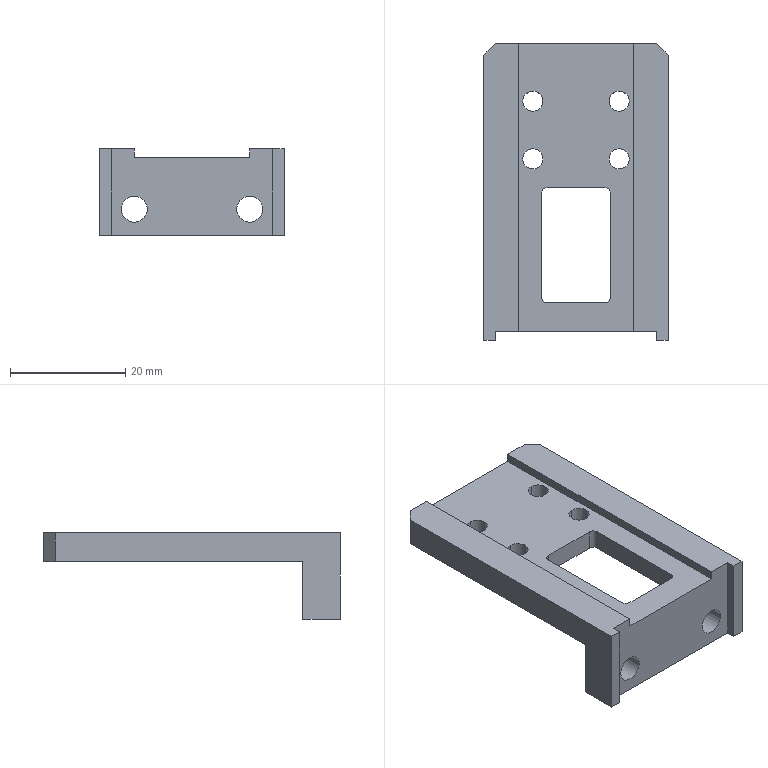Part | STEP file | 11-FG-E04211 | 1 solid | 37 faces | box 32 x 51.5 x 15 mm | volume 7039 mm3 | plane 21 | cylinder 16 | commonest cylinder face diameters 3.5 x8 2 x4 4.5 x4
STEP:
#1=CARTESIAN_POINT('',(12.25,-25.,4.5));
#2=VERTEX_POINT('',#1);
#3=CARTESIAN_POINT('',(7.75,-25.,4.5));
#4=VERTEX_POINT('',#3);
#5=CARTESIAN_POINT('',(10.,-25.,4.5));
#6=DIRECTION('',(0.,1.,0.));
#7=DIRECTION('',(0.,0.,1.));
#8=AXIS2_PLACEMENT_3D('',#5,#6,#7);
#9=CIRCLE('',#8,2.25);
#10=EDGE_CURVE('',#2,#4,#9,.T.);
#11=ORIENTED_EDGE('',*,*,#10,.F.);
#12=CARTESIAN_POINT('',(12.25,-20.,4.5));
#13=VERTEX_POINT('',#12);
#14=CARTESIAN_POINT('',(12.25,-30.,4.5));
#15=DIRECTION('',(0.,1.,0.));
#16=VECTOR('',#15,1000.);
#17=LINE('',#14,#16);
#18=EDGE_CURVE('',#2,#13,#17,.T.);
#19=ORIENTED_EDGE('',*,*,#18,.T.);
#20=CARTESIAN_POINT('',(7.75,-20.,4.5));
#21=VERTEX_POINT('',#20);
#22=CARTESIAN_POINT('',(10.,-20.,4.5));
#23=DIRECTION('',(0.,1.,0.));
#24=DIRECTION('',(-1.,0.,0.));
#25=AXIS2_PLACEMENT_3D('',#22,#23,#24);
#26=CIRCLE('',#25,2.25);
#27=EDGE_CURVE('',#13,#21,#26,.T.);
#28=ORIENTED_EDGE('',*,*,#27,.T.);
#29=CARTESIAN_POINT('',(7.75,-30.,4.5));
#30=DIRECTION('',(0.,1.,0.));
#31=VECTOR('',#30,1000.);
#32=LINE('',#29,#31);
#33=EDGE_CURVE('',#4,#21,#32,.T.);
#34=ORIENTED_EDGE('',*,*,#33,.F.);
#35=EDGE_LOOP('',(#11,#19,#28,#34));
#36=FACE_OUTER_BOUND('',#35,.T.);
#37=CARTESIAN_POINT('',(10.,-30.,4.5));
#38=DIRECTION('',(0.,1.,0.));
#39=DIRECTION('',(-1.,0.,0.));
#40=AXIS2_PLACEMENT_3D('',#37,#38,#39);
#41=CYLINDRICAL_SURFACE('',#40,2.25);
#42=ADVANCED_FACE('',(#36),#41,.F.);
#43=CARTESIAN_POINT('',(-7.75,-25.,4.5));
#44=VERTEX_POINT('',#43);
#45=CARTESIAN_POINT('',(-12.25,-25.,4.5));
#46=VERTEX_POINT('',#45);
#47=CARTESIAN_POINT('',(-10.,-25.,4.5));
#48=DIRECTION('',(0.,1.,0.));
#49=DIRECTION('',(0.,0.,1.));
#50=AXIS2_PLACEMENT_3D('',#47,#48,#49);
#51=CIRCLE('',#50,2.25);
#52=EDGE_CURVE('',#44,#46,#51,.T.);
#53=ORIENTED_EDGE('',*,*,#52,.F.);
#54=CARTESIAN_POINT('',(-7.75,-20.,4.5));
#55=VERTEX_POINT('',#54);
#56=CARTESIAN_POINT('',(-7.75,-30.,4.5));
#57=DIRECTION('',(0.,1.,0.));
#58=VECTOR('',#57,1000.);
#59=LINE('',#56,#58);
#60=EDGE_CURVE('',#44,#55,#59,.T.);
#61=ORIENTED_EDGE('',*,*,#60,.T.);
#62=CARTESIAN_POINT('',(-12.25,-20.,4.5));
#63=VERTEX_POINT('',#62);
#64=CARTESIAN_POINT('',(-10.,-20.,4.5));
#65=DIRECTION('',(0.,1.,0.));
#66=DIRECTION('',(-1.,0.,0.));
#67=AXIS2_PLACEMENT_3D('',#64,#65,#66);
#68=CIRCLE('',#67,2.25);
#69=EDGE_CURVE('',#55,#63,#68,.T.);
#70=ORIENTED_EDGE('',*,*,#69,.T.);
#71=CARTESIAN_POINT('',(-12.25,-30.,4.5));
#72=DIRECTION('',(0.,1.,0.));
#73=VECTOR('',#72,1000.);
#74=LINE('',#71,#73);
#75=EDGE_CURVE('',#46,#63,#74,.T.);
#76=ORIENTED_EDGE('',*,*,#75,.F.);
#77=EDGE_LOOP('',(#53,#61,#70,#76));
#78=FACE_OUTER_BOUND('',#77,.T.);
#79=CARTESIAN_POINT('',(-10.,-30.,4.5));
#80=DIRECTION('',(0.,1.,0.));
#81=DIRECTION('',(-1.,0.,0.));
#82=AXIS2_PLACEMENT_3D('',#79,#80,#81);
#83=CYLINDRICAL_SURFACE('',#82,2.25);
#84=ADVANCED_FACE('',(#78),#83,.F.);
#85=CARTESIAN_POINT('',(-7.5,13.25,13.5));
#86=VERTEX_POINT('',#85);
#87=CARTESIAN_POINT('',(-7.5,16.75,13.5));
#88=VERTEX_POINT('',#87);
#89=CARTESIAN_POINT('',(-7.5,15.,13.5));
#90=DIRECTION('',(0.,0.,-1.));
#91=DIRECTION('',(-1.,0.,0.));
#92=AXIS2_PLACEMENT_3D('',#89,#90,#91);
#93=CIRCLE('',#92,1.75);
#94=EDGE_CURVE('',#86,#88,#93,.T.);
#95=ORIENTED_EDGE('',*,*,#94,.F.);
#96=CARTESIAN_POINT('',(-7.5,13.25,10.));
#97=VERTEX_POINT('',#96);
#98=CARTESIAN_POINT('',(-7.5,13.25,161.));
#99=DIRECTION('',(0.,0.,-1.));
#100=VECTOR('',#99,1000.);
#101=LINE('',#98,#100);
#102=EDGE_CURVE('',#86,#97,#101,.T.);
#103=ORIENTED_EDGE('',*,*,#102,.T.);
#104=CARTESIAN_POINT('',(-7.5,16.75,10.));
#105=VERTEX_POINT('',#104);
#106=CARTESIAN_POINT('',(-7.5,15.,10.));
#107=DIRECTION('',(0.,0.,-1.));
#108=DIRECTION('',(0.,1.,0.));
#109=AXIS2_PLACEMENT_3D('',#106,#107,#108);
#110=CIRCLE('',#109,1.75);
#111=EDGE_CURVE('',#97,#105,#110,.T.);
#112=ORIENTED_EDGE('',*,*,#111,.T.);
#113=CARTESIAN_POINT('',(-7.5,16.75,161.));
#114=DIRECTION('',(0.,0.,-1.));
#115=VECTOR('',#114,1000.);
#116=LINE('',#113,#115);
#117=EDGE_CURVE('',#88,#105,#116,.T.);
#118=ORIENTED_EDGE('',*,*,#117,.F.);
#119=EDGE_LOOP('',(#95,#103,#112,#118));
#120=FACE_OUTER_BOUND('',#119,.T.);
#121=CARTESIAN_POINT('',(-7.5,15.,161.));
#122=DIRECTION('',(0.,0.,-1.));
#123=DIRECTION('',(0.,1.,0.));
#124=AXIS2_PLACEMENT_3D('',#121,#122,#123);
#125=CYLINDRICAL_SURFACE('',#124,1.75);
#126=ADVANCED_FACE('',(#120),#125,.F.);
#127=CARTESIAN_POINT('',(7.5,3.25,13.5));
#128=VERTEX_POINT('',#127);
#129=CARTESIAN_POINT('',(7.5,6.75,13.5));
#130=VERTEX_POINT('',#129);
#131=CARTESIAN_POINT('',(7.5,5.,13.5));
#132=DIRECTION('',(0.,0.,-1.));
#133=DIRECTION('',(-1.,0.,0.));
#134=AXIS2_PLACEMENT_3D('',#131,#132,#133);
#135=CIRCLE('',#134,1.75);
#136=EDGE_CURVE('',#128,#130,#135,.T.);
#137=ORIENTED_EDGE('',*,*,#136,.F.);
#138=CARTESIAN_POINT('',(7.5,3.25,10.));
#139=VERTEX_POINT('',#138);
#140=CARTESIAN_POINT('',(7.5,3.25,161.));
#141=DIRECTION('',(0.,0.,-1.));
#142=VECTOR('',#141,1000.);
#143=LINE('',#140,#142);
#144=EDGE_CURVE('',#128,#139,#143,.T.);
#145=ORIENTED_EDGE('',*,*,#144,.T.);
#146=CARTESIAN_POINT('',(7.5,6.75,10.));
#147=VERTEX_POINT('',#146);
#148=CARTESIAN_POINT('',(7.5,5.,10.));
#149=DIRECTION('',(0.,0.,-1.));
#150=DIRECTION('',(0.,1.,0.));
#151=AXIS2_PLACEMENT_3D('',#148,#149,#150);
#152=CIRCLE('',#151,1.75);
#153=EDGE_CURVE('',#139,#147,#152,.T.);
#154=ORIENTED_EDGE('',*,*,#153,.T.);
#155=CARTESIAN_POINT('',(7.5,6.75,161.));
#156=DIRECTION('',(0.,0.,-1.));
#157=VECTOR('',#156,1000.);
#158=LINE('',#155,#157);
#159=EDGE_CURVE('',#130,#147,#158,.T.);
#160=ORIENTED_EDGE('',*,*,#159,.F.);
#161=EDGE_LOOP('',(#137,#145,#154,#160));
#162=FACE_OUTER_BOUND('',#161,.T.);
#163=CARTESIAN_POINT('',(7.5,5.,161.));
#164=DIRECTION('',(0.,0.,-1.));
#165=DIRECTION('',(0.,1.,0.));
#166=AXIS2_PLACEMENT_3D('',#163,#164,#165);
#167=CYLINDRICAL_SURFACE('',#166,1.75);
#168=ADVANCED_FACE('',(#162),#167,.F.);
#169=CARTESIAN_POINT('',(-7.5,3.25,13.5));
#170=VERTEX_POINT('',#169);
#171=CARTESIAN_POINT('',(-7.5,6.75,13.5));
#172=VERTEX_POINT('',#171);
#173=CARTESIAN_POINT('',(-7.5,5.,13.5));
#174=DIRECTION('',(0.,0.,-1.));
#175=DIRECTION('',(-1.,0.,0.));
#176=AXIS2_PLACEMENT_3D('',#173,#174,#175);
#177=CIRCLE('',#176,1.75);
#178=EDGE_CURVE('',#170,#172,#177,.T.);
#179=ORIENTED_EDGE('',*,*,#178,.F.);
#180=CARTESIAN_POINT('',(-7.5,3.25,10.));
#181=VERTEX_POINT('',#180);
#182=CARTESIAN_POINT('',(-7.5,3.25,161.));
#183=DIRECTION('',(0.,0.,-1.));
#184=VECTOR('',#183,1000.);
#185=LINE('',#182,#184);
#186=EDGE_CURVE('',#170,#181,#185,.T.);
#187=ORIENTED_EDGE('',*,*,#186,.T.);
#188=CARTESIAN_POINT('',(-7.5,6.75,10.));
#189=VERTEX_POINT('',#188);
#190=CARTESIAN_POINT('',(-7.5,5.,10.));
#191=DIRECTION('',(0.,0.,-1.));
#192=DIRECTION('',(0.,1.,0.));
#193=AXIS2_PLACEMENT_3D('',#190,#191,#192);
#194=CIRCLE('',#193,1.75);
#195=EDGE_CURVE('',#181,#189,#194,.T.);
#196=ORIENTED_EDGE('',*,*,#195,.T.);
#197=CARTESIAN_POINT('',(-7.5,6.75,161.));
#198=DIRECTION('',(0.,0.,-1.));
#199=VECTOR('',#198,1000.);
#200=LINE('',#197,#199);
#201=EDGE_CURVE('',#172,#189,#200,.T.);
#202=ORIENTED_EDGE('',*,*,#201,.F.);
#203=EDGE_LOOP('',(#179,#187,#196,#202));
#204=FACE_OUTER_BOUND('',#203,.T.);
#205=CARTESIAN_POINT('',(-7.5,5.,161.));
#206=DIRECTION('',(0.,0.,-1.));
#207=DIRECTION('',(0.,1.,0.));
#208=AXIS2_PLACEMENT_3D('',#205,#206,#207);
#209=CYLINDRICAL_SURFACE('',#208,1.75);
#210=ADVANCED_FACE('',(#204),#209,.F.);
#211=CARTESIAN_POINT('',(7.5,13.25,13.5));
#212=VERTEX_POINT('',#211);
#213=CARTESIAN_POINT('',(7.5,16.75,13.5));
#214=VERTEX_POINT('',#213);
#215=CARTESIAN_POINT('',(7.5,15.,13.5));
#216=DIRECTION('',(0.,0.,-1.));
#217=DIRECTION('',(-1.,0.,0.));
#218=AXIS2_PLACEMENT_3D('',#215,#216,#217);
#219=CIRCLE('',#218,1.75);
#220=EDGE_CURVE('',#212,#214,#219,.T.);
#221=ORIENTED_EDGE('',*,*,#220,.F.);
#222=CARTESIAN_POINT('',(7.5,13.25,10.));
#223=VERTEX_POINT('',#222);
#224=CARTESIAN_POINT('',(7.5,13.25,161.));
#225=DIRECTION('',(0.,0.,-1.));
#226=VECTOR('',#225,1000.);
#227=LINE('',#224,#226);
#228=EDGE_CURVE('',#212,#223,#227,.T.);
#229=ORIENTED_EDGE('',*,*,#228,.T.);
#230=CARTESIAN_POINT('',(7.5,16.75,10.));
#231=VERTEX_POINT('',#230);
#232=CARTESIAN_POINT('',(7.5,15.,10.));
#233=DIRECTION('',(0.,0.,-1.));
#234=DIRECTION('',(0.,1.,0.));
#235=AXIS2_PLACEMENT_3D('',#232,#233,#234);
#236=CIRCLE('',#235,1.75);
#237=EDGE_CURVE('',#223,#231,#236,.T.);
#238=ORIENTED_EDGE('',*,*,#237,.T.);
#239=CARTESIAN_POINT('',(7.5,16.75,161.));
#240=DIRECTION('',(0.,0.,-1.));
#241=VECTOR('',#240,1000.);
#242=LINE('',#239,#241);
#243=EDGE_CURVE('',#214,#231,#242,.T.);
#244=ORIENTED_EDGE('',*,*,#243,.F.);
#245=EDGE_LOOP('',(#221,#229,#238,#244));
#246=FACE_OUTER_BOUND('',#245,.T.);
#247=CARTESIAN_POINT('',(7.5,15.,161.));
#248=DIRECTION('',(0.,0.,-1.));
#249=DIRECTION('',(0.,1.,0.));
#250=AXIS2_PLACEMENT_3D('',#247,#248,#249);
#251=CYLINDRICAL_SURFACE('',#250,1.75);
#252=ADVANCED_FACE('',(#246),#251,.F.);
#253=CARTESIAN_POINT('',(10.,-25.,4.5));
#254=DIRECTION('',(0.,1.,0.));
#255=DIRECTION('',(0.,0.,1.));
#256=AXIS2_PLACEMENT_3D('',#253,#254,#255);
#257=CIRCLE('',#256,2.25);
#258=EDGE_CURVE('',#4,#2,#257,.T.);
#259=ORIENTED_EDGE('',*,*,#258,.T.);
#260=ORIENTED_EDGE('',*,*,#10,.T.);
#261=EDGE_LOOP('',(#259,#260));
#262=FACE_BOUND('',#261,.T.);
#263=CARTESIAN_POINT('',(-10.,-25.,4.5));
#264=DIRECTION('',(0.,1.,0.));
#265=DIRECTION('',(0.,0.,1.));
#266=AXIS2_PLACEMENT_3D('',#263,#264,#265);
#267=CIRCLE('',#266,2.25);
#268=EDGE_CURVE('',#46,#44,#267,.T.);
#269=ORIENTED_EDGE('',*,*,#268,.T.);
#270=ORIENTED_EDGE('',*,*,#52,.T.);
#271=EDGE_LOOP('',(#269,#270));
#272=FACE_BOUND('',#271,.T.);
#273=CARTESIAN_POINT('',(-14.,-25.,15.));
#274=VERTEX_POINT('',#273);
#275=CARTESIAN_POINT('',(-10.,-25.,15.));
#276=VERTEX_POINT('',#275);
#277=CARTESIAN_POINT('',(-16.,-25.,15.));
#278=DIRECTION('',(1.,0.,0.));
#279=VECTOR('',#278,1000.);
#280=LINE('',#277,#279);
#281=EDGE_CURVE('',#274,#276,#280,.T.);
#282=ORIENTED_EDGE('',*,*,#281,.F.);
#283=CARTESIAN_POINT('',(-14.,-25.,0.));
#284=VERTEX_POINT('',#283);
#285=CARTESIAN_POINT('',(-14.,-25.,17.5));
#286=DIRECTION('',(0.,0.,-1.));
#287=VECTOR('',#286,1000.);
#288=LINE('',#285,#287);
#289=EDGE_CURVE('',#274,#284,#288,.T.);
#290=ORIENTED_EDGE('',*,*,#289,.T.);
#291=CARTESIAN_POINT('',(14.,-25.,0.));
#292=VERTEX_POINT('',#291);
#293=CARTESIAN_POINT('',(-16.,-25.,0.));
#294=DIRECTION('',(1.,0.,0.));
#295=VECTOR('',#294,1000.);
#296=LINE('',#293,#295);
#297=EDGE_CURVE('',#284,#292,#296,.T.);
#298=ORIENTED_EDGE('',*,*,#297,.T.);
#299=CARTESIAN_POINT('',(14.,-25.,15.));
#300=VERTEX_POINT('',#299);
#301=CARTESIAN_POINT('',(14.,-25.,17.5));
#302=DIRECTION('',(0.,0.,-1.));
#303=VECTOR('',#302,1000.);
#304=LINE('',#301,#303);
#305=EDGE_CURVE('',#300,#292,#304,.T.);
#306=ORIENTED_EDGE('',*,*,#305,.F.);
#307=CARTESIAN_POINT('',(10.,-25.,15.));
#308=VERTEX_POINT('',#307);
#309=CARTESIAN_POINT('',(-16.,-25.,15.));
#310=DIRECTION('',(1.,0.,0.));
#311=VECTOR('',#310,1000.);
#312=LINE('',#309,#311);
#313=EDGE_CURVE('',#308,#300,#312,.T.);
#314=ORIENTED_EDGE('',*,*,#313,.F.);
#315=CARTESIAN_POINT('',(10.,-25.,13.5));
#316=VERTEX_POINT('',#315);
#317=CARTESIAN_POINT('',(10.,-25.,15.));
#318=DIRECTION('',(0.,0.,-1.));
#319=VECTOR('',#318,1000.);
#320=LINE('',#317,#319);
#321=EDGE_CURVE('',#308,#316,#320,.T.);
#322=ORIENTED_EDGE('',*,*,#321,.T.);
#323=CARTESIAN_POINT('',(-10.,-25.,13.5));
#324=VERTEX_POINT('',#323);
#325=CARTESIAN_POINT('',(-16.,-25.,13.5));
#326=DIRECTION('',(-1.,0.,0.));
#327=VECTOR('',#326,1000.);
#328=LINE('',#325,#327);
#329=EDGE_CURVE('',#316,#324,#328,.T.);
#330=ORIENTED_EDGE('',*,*,#329,.T.);
#331=CARTESIAN_POINT('',(-10.,-25.,15.));
#332=DIRECTION('',(0.,0.,1.));
#333=VECTOR('',#332,1000.);
#334=LINE('',#331,#333);
#335=EDGE_CURVE('',#324,#276,#334,.T.);
#336=ORIENTED_EDGE('',*,*,#335,.T.);
#337=EDGE_LOOP('',(#282,#290,#298,#306,#314,#322,#330,#336));
#338=FACE_OUTER_BOUND('',#337,.T.);
#339=CARTESIAN_POINT('',(-16.,-25.,15.));
#340=DIRECTION('',(0.,1.,0.));
#341=DIRECTION('',(0.,0.,1.));
#342=AXIS2_PLACEMENT_3D('',#339,#340,#341);
#343=PLANE('',#342);
#344=ADVANCED_FACE('',(#262,#272,#338),#343,.F.);
#345=CARTESIAN_POINT('',(16.,-26.5,15.));
#346=VERTEX_POINT('',#345);
#347=CARTESIAN_POINT('',(16.,23.,15.));
#348=VERTEX_POINT('',#347);
#349=CARTESIAN_POINT('',(16.,25.,15.));
#350=DIRECTION('',(0.,1.,0.));
#351=VECTOR('',#350,1000.);
#352=LINE('',#349,#351);
#353=EDGE_CURVE('',#346,#348,#352,.T.);
#354=ORIENTED_EDGE('',*,*,#353,.T.);
#355=CARTESIAN_POINT('',(14.,25.,15.));
#356=VERTEX_POINT('',#355);
#357=CARTESIAN_POINT('',(19.5,19.5,15.));
#358=DIRECTION('',(-0.7071,0.7071,0.));
#359=VECTOR('',#358,1000.);
#360=LINE('',#357,#359);
#361=EDGE_CURVE('',#348,#356,#360,.T.);
#362=ORIENTED_EDGE('',*,*,#361,.T.);
#363=CARTESIAN_POINT('',(10.,25.,15.));
#364=VERTEX_POINT('',#363);
#365=CARTESIAN_POINT('',(-16.,25.,15.));
#366=DIRECTION('',(-1.,0.,0.));
#367=VECTOR('',#366,1000.);
#368=LINE('',#365,#367);
#369=EDGE_CURVE('',#356,#364,#368,.T.);
#370=ORIENTED_EDGE('',*,*,#369,.T.);
#371=CARTESIAN_POINT('',(10.,0.,15.));
#372=DIRECTION('',(0.,1.,0.));
#373=VECTOR('',#372,1000.);
#374=LINE('',#371,#373);
#375=EDGE_CURVE('',#308,#364,#374,.T.);
#376=ORIENTED_EDGE('',*,*,#375,.F.);
#377=ORIENTED_EDGE('',*,*,#313,.T.);
#378=CARTESIAN_POINT('',(14.,-26.5,15.));
#379=VERTEX_POINT('',#378);
#380=CARTESIAN_POINT('',(14.,-25.,15.));
#381=DIRECTION('',(0.,1.,0.));
#382=VECTOR('',#381,1000.);
#383=LINE('',#380,#382);
#384=EDGE_CURVE('',#379,#300,#383,.T.);
#385=ORIENTED_EDGE('',*,*,#384,.F.);
#386=CARTESIAN_POINT('',(16.,-26.5,15.));
#387=DIRECTION('',(-1.,0.,0.));
#388=VECTOR('',#387,1000.);
#389=LINE('',#386,#388);
#390=EDGE_CURVE('',#346,#379,#389,.T.);
#391=ORIENTED_EDGE('',*,*,#390,.F.);
#392=EDGE_LOOP('',(#354,#362,#370,#376,#377,#385,#391));
#393=FACE_OUTER_BOUND('',#392,.T.);
#394=CARTESIAN_POINT('',(0.,0.,15.));
#395=DIRECTION('',(0.,0.,1.));
#396=DIRECTION('',(1.,0.,0.));
#397=AXIS2_PLACEMENT_3D('',#394,#395,#396);
#398=PLANE('',#397);
#399=ADVANCED_FACE('',(#393),#398,.T.);
#400=CARTESIAN_POINT('',(16.,-20.,10.));
#401=VERTEX_POINT('',#400);
#402=CARTESIAN_POINT('',(16.,23.,10.));
#403=VERTEX_POINT('',#402);
#404=CARTESIAN_POINT('',(16.,25.,10.));
#405=DIRECTION('',(0.,1.,0.));
#406=VECTOR('',#405,1000.);
#407=LINE('',#404,#406);
#408=EDGE_CURVE('',#401,#403,#407,.T.);
#409=ORIENTED_EDGE('',*,*,#408,.T.);
#410=CARTESIAN_POINT('',(16.,23.,15.));
#411=DIRECTION('',(0.,0.,1.));
#412=VECTOR('',#411,1000.);
#413=LINE('',#410,#412);
#414=EDGE_CURVE('',#403,#348,#413,.T.);
#415=ORIENTED_EDGE('',*,*,#414,.T.);
#416=ORIENTED_EDGE('',*,*,#353,.F.);
#417=CARTESIAN_POINT('',(16.,-26.5,0.));
#418=VERTEX_POINT('',#417);
#419=CARTESIAN_POINT('',(16.,-26.5,17.5));
#420=DIRECTION('',(0.,0.,-1.));
#421=VECTOR('',#420,1000.);
#422=LINE('',#419,#421);
#423=EDGE_CURVE('',#346,#418,#422,.T.);
#424=ORIENTED_EDGE('',*,*,#423,.T.);
#425=CARTESIAN_POINT('',(16.,-20.,0.));
#426=VERTEX_POINT('',#425);
#427=CARTESIAN_POINT('',(16.,25.,0.));
#428=DIRECTION('',(0.,1.,0.));
#429=VECTOR('',#428,1000.);
#430=LINE('',#427,#429);
#431=EDGE_CURVE('',#418,#426,#430,.T.);
#432=ORIENTED_EDGE('',*,*,#431,.T.);
#433=CARTESIAN_POINT('',(16.,-20.,15.));
#434=DIRECTION('',(0.,0.,1.));
#435=VECTOR('',#434,1000.);
#436=LINE('',#433,#435);
#437=EDGE_CURVE('',#426,#401,#436,.T.);
#438=ORIENTED_EDGE('',*,*,#437,.T.);
#439=EDGE_LOOP('',(#409,#415,#416,#424,#432,#438));
#440=FACE_OUTER_BOUND('',#439,.T.);
#441=CARTESIAN_POINT('',(16.,25.,15.));
#442=DIRECTION('',(-1.,0.,0.));
#443=DIRECTION('',(0.,-1.,0.));
#444=AXIS2_PLACEMENT_3D('',#441,#442,#443);
#445=PLANE('',#444);
#446=ADVANCED_FACE('',(#440),#445,.F.);
#447=CARTESIAN_POINT('',(14.,25.,10.));
#448=VERTEX_POINT('',#447);
#449=CARTESIAN_POINT('',(-14.,25.,10.));
#450=VERTEX_POINT('',#449);
#451=CARTESIAN_POINT('',(135.,25.,10.));
#452=DIRECTION('',(-1.,0.,0.));
#453=VECTOR('',#452,1000.);
#454=LINE('',#451,#453);
#455=EDGE_CURVE('',#448,#450,#454,.T.);
#456=ORIENTED_EDGE('',*,*,#455,.T.);
#457=CARTESIAN_POINT('',(-14.,25.,15.));
#458=VERTEX_POINT('',#457);
#459=CARTESIAN_POINT('',(-14.,25.,15.));
#460=DIRECTION('',(0.,0.,1.));
#461=VECTOR('',#460,1000.);
#462=LINE('',#459,#461);
#463=EDGE_CURVE('',#450,#458,#462,.T.);
#464=ORIENTED_EDGE('',*,*,#463,.T.);
#465=CARTESIAN_POINT('',(-10.,25.,15.));
#466=VERTEX_POINT('',#465);
#467=CARTESIAN_POINT('',(-16.,25.,15.));
#468=DIRECTION('',(-1.,0.,0.));
#469=VECTOR('',#468,1000.);
#470=LINE('',#467,#469);
#471=EDGE_CURVE('',#466,#458,#470,.T.);
#472=ORIENTED_EDGE('',*,*,#471,.F.);
#473=CARTESIAN_POINT('',(-10.,25.,13.5));
#474=VERTEX_POINT('',#473);
#475=CARTESIAN_POINT('',(-10.,25.,15.));
#476=DIRECTION('',(0.,0.,1.));
#477=VECTOR('',#476,1000.);
#478=LINE('',#475,#477);
#479=EDGE_CURVE('',#474,#466,#478,.T.);
#480=ORIENTED_EDGE('',*,*,#479,.F.);
#481=CARTESIAN_POINT('',(10.,25.,13.5));
#482=VERTEX_POINT('',#481);
#483=CARTESIAN_POINT('',(10.,25.,13.5));
#484=DIRECTION('',(-1.,0.,0.));
#485=VECTOR('',#484,1000.);
#486=LINE('',#483,#485);
#487=EDGE_CURVE('',#482,#474,#486,.T.);
#488=ORIENTED_EDGE('',*,*,#487,.F.);
#489=CARTESIAN_POINT('',(10.,25.,15.));
#490=DIRECTION('',(0.,0.,-1.));
#491=VECTOR('',#490,1000.);
#492=LINE('',#489,#491);
#493=EDGE_CURVE('',#364,#482,#492,.T.);
#494=ORIENTED_EDGE('',*,*,#493,.F.);
#495=ORIENTED_EDGE('',*,*,#369,.F.);
#496=CARTESIAN_POINT('',(14.,25.,15.));
#497=DIRECTION('',(0.,0.,-1.));
#498=VECTOR('',#497,1000.);
#499=LINE('',#496,#498);
#500=EDGE_CURVE('',#356,#448,#499,.T.);
#501=ORIENTED_EDGE('',*,*,#500,.T.);
#502=EDGE_LOOP('',(#456,#464,#472,#480,#488,#494,#495,#501));
#503=FACE_OUTER_BOUND('',#502,.T.);
#504=CARTESIAN_POINT('',(-16.,25.,15.));
#505=DIRECTION('',(0.,-1.,0.));
#506=DIRECTION('',(0.,0.,-1.));
#507=AXIS2_PLACEMENT_3D('',#504,#505,#506);
#508=PLANE('',#507);
#509=ADVANCED_FACE('',(#503),#508,.F.);
#510=CARTESIAN_POINT('',(-16.,23.,15.));
#511=VERTEX_POINT('',#510);
#512=CARTESIAN_POINT('',(-16.,-26.5,15.));
#513=VERTEX_POINT('',#512);
#514=CARTESIAN_POINT('',(-16.,25.,15.));
#515=DIRECTION('',(0.,-1.,0.));
#516=VECTOR('',#515,1000.);
#517=LINE('',#514,#516);
#518=EDGE_CURVE('',#511,#513,#517,.T.);
#519=ORIENTED_EDGE('',*,*,#518,.F.);
#520=CARTESIAN_POINT('',(-16.,23.,10.));
#521=VERTEX_POINT('',#520);
#522=CARTESIAN_POINT('',(-16.,23.,15.));
#523=DIRECTION('',(0.,0.,-1.));
#524=VECTOR('',#523,1000.);
#525=LINE('',#522,#524);
#526=EDGE_CURVE('',#511,#521,#525,.T.);
#527=ORIENTED_EDGE('',*,*,#526,.T.);
#528=CARTESIAN_POINT('',(-16.,-20.,10.));
#529=VERTEX_POINT('',#528);
#530=CARTESIAN_POINT('',(-16.,25.,10.));
#531=DIRECTION('',(0.,1.,0.));
#532=VECTOR('',#531,1000.);
#533=LINE('',#530,#532);
#534=EDGE_CURVE('',#529,#521,#533,.T.);
#535=ORIENTED_EDGE('',*,*,#534,.F.);
#536=CARTESIAN_POINT('',(-16.,-20.,0.));
#537=VERTEX_POINT('',#536);
#538=CARTESIAN_POINT('',(-16.,-20.,0.));
#539=DIRECTION('',(0.,0.,1.));
#540=VECTOR('',#539,1000.);
#541=LINE('',#538,#540);
#542=EDGE_CURVE('',#537,#529,#541,.T.);
#543=ORIENTED_EDGE('',*,*,#542,.F.);
#544=CARTESIAN_POINT('',(-16.,-26.5,0.));
#545=VERTEX_POINT('',#544);
#546=CARTESIAN_POINT('',(-16.,25.,0.));
#547=DIRECTION('',(0.,-1.,0.));
#548=VECTOR('',#547,1000.);
#549=LINE('',#546,#548);
#550=EDGE_CURVE('',#537,#545,#549,.T.);
#551=ORIENTED_EDGE('',*,*,#550,.T.);
#552=CARTESIAN_POINT('',(-16.,-26.5,17.5));
#553=DIRECTION('',(0.,0.,-1.));
#554=VECTOR('',#553,1000.);
#555=LINE('',#552,#554);
#556=EDGE_CURVE('',#513,#545,#555,.T.);
#557=ORIENTED_EDGE('',*,*,#556,.F.);
#558=EDGE_LOOP('',(#519,#527,#535,#543,#551,#557));
#559=FACE_OUTER_BOUND('',#558,.T.);
#560=CARTESIAN_POINT('',(-16.,25.,15.));
#561=DIRECTION('',(1.,0.,0.));
#562=DIRECTION('',(0.,1.,0.));
#563=AXIS2_PLACEMENT_3D('',#560,#561,#562);
#564=PLANE('',#563);
#565=ADVANCED_FACE('',(#559),#564,.F.);
#566=ORIENTED_EDGE('',*,*,#471,.T.);
#567=CARTESIAN_POINT('',(-19.5,19.5,15.));
#568=DIRECTION('',(-0.7071,-0.7071,0.));
#569=VECTOR('',#568,1000.);
#570=LINE('',#567,#569);
#571=EDGE_CURVE('',#458,#511,#570,.T.);
#572=ORIENTED_EDGE('',*,*,#571,.T.);
#573=ORIENTED_EDGE('',*,*,#518,.T.);
#574=CARTESIAN_POINT('',(-14.,-26.5,15.));
#575=VERTEX_POINT('',#574);
#576=CARTESIAN_POINT('',(-16.,-26.5,15.));
#577=DIRECTION('',(-1.,0.,0.));
#578=VECTOR('',#577,1000.);
#579=LINE('',#576,#578);
#580=EDGE_CURVE('',#575,#513,#579,.T.);
#581=ORIENTED_EDGE('',*,*,#580,.F.);
#582=CARTESIAN_POINT('',(-14.,-25.,15.));
#583=DIRECTION('',(0.,-1.,0.));
#584=VECTOR('',#583,1000.);
#585=LINE('',#582,#584);
#586=EDGE_CURVE('',#274,#575,#585,.T.);
#587=ORIENTED_EDGE('',*,*,#586,.F.);
#588=ORIENTED_EDGE('',*,*,#281,.T.);
#589=CARTESIAN_POINT('',(-10.,0.,15.));
#590=DIRECTION('',(0.,-1.,0.));
#591=VECTOR('',#590,1000.);
#592=LINE('',#589,#591);
#593=EDGE_CURVE('',#466,#276,#592,.T.);
#594=ORIENTED_EDGE('',*,*,#593,.F.);
#595=EDGE_LOOP('',(#566,#572,#573,#581,#587,#588,#594));
#596=FACE_OUTER_BOUND('',#595,.T.);
#597=CARTESIAN_POINT('',(0.,0.,15.));
#598=DIRECTION('',(0.,0.,1.));
#599=DIRECTION('',(1.,0.,0.));
#600=AXIS2_PLACEMENT_3D('',#597,#598,#599);
#601=PLANE('',#600);
#602=ADVANCED_FACE('',(#596),#601,.T.);
#603=ORIENTED_EDGE('',*,*,#550,.F.);
#604=CARTESIAN_POINT('',(0.,-20.,0.));
#605=DIRECTION('',(1.,0.,0.));
#606=VECTOR('',#605,1000.);
#607=LINE('',#604,#606);
#608=EDGE_CURVE('',#537,#426,#607,.T.);
#609=ORIENTED_EDGE('',*,*,#608,.T.);
#610=ORIENTED_EDGE('',*,*,#431,.F.);
#611=CARTESIAN_POINT('',(14.,-26.5,0.));
#612=VERTEX_POINT('',#611);
#613=CARTESIAN_POINT('',(16.,-26.5,0.));
#614=DIRECTION('',(-1.,0.,0.));
#615=VECTOR('',#614,1000.);
#616=LINE('',#613,#615);
#617=EDGE_CURVE('',#418,#612,#616,.T.);
#618=ORIENTED_EDGE('',*,*,#617,.T.);
#619=CARTESIAN_POINT('',(14.,-25.,0.));
#620=DIRECTION('',(0.,1.,0.));
#621=VECTOR('',#620,1000.);
#622=LINE('',#619,#621);
#623=EDGE_CURVE('',#612,#292,#622,.T.);
#624=ORIENTED_EDGE('',*,*,#623,.T.);
#625=ORIENTED_EDGE('',*,*,#297,.F.);
#626=CARTESIAN_POINT('',(-14.,-26.5,0.));
#627=VERTEX_POINT('',#626);
#628=CARTESIAN_POINT('',(-14.,-25.,0.));
#629=DIRECTION('',(0.,-1.,0.));
#630=VECTOR('',#629,1000.);
#631=LINE('',#628,#630);
#632=EDGE_CURVE('',#284,#627,#631,.T.);
#633=ORIENTED_EDGE('',*,*,#632,.T.);
#634=CARTESIAN_POINT('',(-16.,-26.5,0.));
#635=DIRECTION('',(-1.,0.,0.));
#636=VECTOR('',#635,1000.);
#637=LINE('',#634,#636);
#638=EDGE_CURVE('',#627,#545,#637,.T.);
#639=ORIENTED_EDGE('',*,*,#638,.T.);
#640=EDGE_LOOP('',(#603,#609,#610,#618,#624,#625,#633,#639));
#641=FACE_OUTER_BOUND('',#640,.T.);
#642=CARTESIAN_POINT('',(0.,0.,0.));
#643=DIRECTION('',(0.,0.,1.));
#644=DIRECTION('',(1.,0.,0.));
#645=AXIS2_PLACEMENT_3D('',#642,#643,#644);
#646=PLANE('',#645);
#647=ADVANCED_FACE('',(#641),#646,.F.);
#648=CARTESIAN_POINT('',(6.,-1.,13.5));
#649=VERTEX_POINT('',#648);
#650=CARTESIAN_POINT('',(6.,-19.,13.5));
#651=VERTEX_POINT('',#650);
#652=CARTESIAN_POINT('',(6.,-126.,13.5));
#653=DIRECTION('',(0.,-1.,0.));
#654=VECTOR('',#653,1000.);
#655=LINE('',#652,#654);
#656=EDGE_CURVE('',#649,#651,#655,.T.);
#657=ORIENTED_EDGE('',*,*,#656,.T.);
#658=CARTESIAN_POINT('',(5.,-20.,13.5));
#659=VERTEX_POINT('',#658);
#660=CARTESIAN_POINT('',(5.,-19.,13.5));
#661=DIRECTION('',(0.,0.,-1.));
#662=DIRECTION('',(-1.,0.,0.));
#663=AXIS2_PLACEMENT_3D('',#660,#661,#662);
#664=CIRCLE('',#663,1.);
#665=EDGE_CURVE('',#651,#659,#664,.T.);
#666=ORIENTED_EDGE('',*,*,#665,.T.);
#667=CARTESIAN_POINT('',(-5.,-20.,13.5));
#668=VERTEX_POINT('',#667);
#669=CARTESIAN_POINT('',(10.,-20.,13.5));
#670=DIRECTION('',(-1.,0.,0.));
#671=VECTOR('',#670,1000.);
#672=LINE('',#669,#671);
#673=EDGE_CURVE('',#659,#668,#672,.T.);
#674=ORIENTED_EDGE('',*,*,#673,.T.);
#675=CARTESIAN_POINT('',(-6.,-19.,13.5));
#676=VERTEX_POINT('',#675);
#677=CARTESIAN_POINT('',(-5.,-19.,13.5));
#678=DIRECTION('',(0.,0.,-1.));
#679=DIRECTION('',(-1.,0.,0.));
#680=AXIS2_PLACEMENT_3D('',#677,#678,#679);
#681=CIRCLE('',#680,1.);
#682=EDGE_CURVE('',#668,#676,#681,.T.);
#683=ORIENTED_EDGE('',*,*,#682,.T.);
#684=CARTESIAN_POINT('',(-6.,-1.,13.5));
#685=VERTEX_POINT('',#684);
#686=CARTESIAN_POINT('',(-6.,-126.,13.5));
#687=DIRECTION('',(0.,1.,0.));
#688=VECTOR('',#687,1000.);
#689=LINE('',#686,#688);
#690=EDGE_CURVE('',#676,#685,#689,.T.);
#691=ORIENTED_EDGE('',*,*,#690,.T.);
#692=CARTESIAN_POINT('',(-5.,0.,13.5));
#693=VERTEX_POINT('',#692);
#694=CARTESIAN_POINT('',(-5.,-1.,13.5));
#695=DIRECTION('',(0.,0.,-1.));
#696=DIRECTION('',(-1.,0.,0.));
#697=AXIS2_PLACEMENT_3D('',#694,#695,#696);
#698=CIRCLE('',#697,1.);
#699=EDGE_CURVE('',#685,#693,#698,.T.);
#700=ORIENTED_EDGE('',*,*,#699,.T.);
#701=CARTESIAN_POINT('',(5.,0.,13.5));
#702=VERTEX_POINT('',#701);
#703=CARTESIAN_POINT('',(10.,0.,13.5));
#704=DIRECTION('',(1.,0.,0.));
#705=VECTOR('',#704,1000.);
#706=LINE('',#703,#705);
#707=EDGE_CURVE('',#693,#702,#706,.T.);
#708=ORIENTED_EDGE('',*,*,#707,.T.);
#709=CARTESIAN_POINT('',(5.,-1.,13.5));
#710=DIRECTION('',(0.,0.,-1.));
#711=DIRECTION('',(-1.,0.,0.));
#712=AXIS2_PLACEMENT_3D('',#709,#710,#711);
#713=CIRCLE('',#712,1.);
#714=EDGE_CURVE('',#702,#649,#713,.T.);
#715=ORIENTED_EDGE('',*,*,#714,.T.);
#716=EDGE_LOOP('',(#657,#666,#674,#683,#691,#700,#708,#715));
#717=FACE_BOUND('',#716,.T.);
#718=CARTESIAN_POINT('',(-7.5,15.,13.5));
#719=DIRECTION('',(0.,0.,-1.));
#720=DIRECTION('',(-1.,0.,0.));
#721=AXIS2_PLACEMENT_3D('',#718,#719,#720);
#722=CIRCLE('',#721,1.75);
#723=EDGE_CURVE('',#88,#86,#722,.T.);
#724=ORIENTED_EDGE('',*,*,#723,.T.);
#725=ORIENTED_EDGE('',*,*,#94,.T.);
#726=EDGE_LOOP('',(#724,#725));
#727=FACE_BOUND('',#726,.T.);
#728=CARTESIAN_POINT('',(7.5,5.,13.5));
#729=DIRECTION('',(0.,0.,-1.));
#730=DIRECTION('',(-1.,0.,0.));
#731=AXIS2_PLACEMENT_3D('',#728,#729,#730);
#732=CIRCLE('',#731,1.75);
#733=EDGE_CURVE('',#130,#128,#732,.T.);
#734=ORIENTED_EDGE('',*,*,#733,.T.);
#735=ORIENTED_EDGE('',*,*,#136,.T.);
#736=EDGE_LOOP('',(#734,#735));
#737=FACE_BOUND('',#736,.T.);
#738=CARTESIAN_POINT('',(-7.5,5.,13.5));
#739=DIRECTION('',(0.,0.,-1.));
#740=DIRECTION('',(-1.,0.,0.));
#741=AXIS2_PLACEMENT_3D('',#738,#739,#740);
#742=CIRCLE('',#741,1.75);
#743=EDGE_CURVE('',#172,#170,#742,.T.);
#744=ORIENTED_EDGE('',*,*,#743,.T.);
#745=ORIENTED_EDGE('',*,*,#178,.T.);
#746=EDGE_LOOP('',(#744,#745));
#747=FACE_BOUND('',#746,.T.);
#748=CARTESIAN_POINT('',(7.5,15.,13.5));
#749=DIRECTION('',(0.,0.,-1.));
#750=DIRECTION('',(-1.,0.,0.));
#751=AXIS2_PLACEMENT_3D('',#748,#749,#750);
#752=CIRCLE('',#751,1.75);
#753=EDGE_CURVE('',#214,#212,#752,.T.);
#754=ORIENTED_EDGE('',*,*,#753,.T.);
#755=ORIENTED_EDGE('',*,*,#220,.T.);
#756=EDGE_LOOP('',(#754,#755));
#757=FACE_BOUND('',#756,.T.);
#758=CARTESIAN_POINT('',(10.,-126.,13.5));
#759=DIRECTION('',(0.,1.,0.));
#760=VECTOR('',#759,1000.);
#761=LINE('',#758,#760);
#762=EDGE_CURVE('',#316,#482,#761,.T.);
#763=ORIENTED_EDGE('',*,*,#762,.T.);
#764=ORIENTED_EDGE('',*,*,#487,.T.);
#765=CARTESIAN_POINT('',(-10.,-126.,13.5));
#766=DIRECTION('',(0.,1.,0.));
#767=VECTOR('',#766,1000.);
#768=LINE('',#765,#767);
#769=EDGE_CURVE('',#324,#474,#768,.T.);
#770=ORIENTED_EDGE('',*,*,#769,.F.);
#771=ORIENTED_EDGE('',*,*,#329,.F.);
#772=EDGE_LOOP('',(#763,#764,#770,#771));
#773=FACE_OUTER_BOUND('',#772,.T.);
#774=CARTESIAN_POINT('',(10.,-126.,13.5));
#775=DIRECTION('',(0.,0.,-1.));
#776=DIRECTION('',(-1.,0.,0.));
#777=AXIS2_PLACEMENT_3D('',#774,#775,#776);
#778=PLANE('',#777);
#779=ADVANCED_FACE('',(#717,#727,#737,#747,#757,#773),#778,.F.);
#780=ORIENTED_EDGE('',*,*,#375,.T.);
#781=ORIENTED_EDGE('',*,*,#493,.T.);
#782=ORIENTED_EDGE('',*,*,#762,.F.);
#783=ORIENTED_EDGE('',*,*,#321,.F.);
#784=EDGE_LOOP('',(#780,#781,#782,#783));
#785=FACE_OUTER_BOUND('',#784,.T.);
#786=CARTESIAN_POINT('',(10.,-126.,15.));
#787=DIRECTION('',(1.,0.,0.));
#788=DIRECTION('',(0.,0.,-1.));
#789=AXIS2_PLACEMENT_3D('',#786,#787,#788);
#790=PLANE('',#789);
#791=ADVANCED_FACE('',(#785),#790,.F.);
#792=ORIENTED_EDGE('',*,*,#769,.T.);
#793=ORIENTED_EDGE('',*,*,#479,.T.);
#794=ORIENTED_EDGE('',*,*,#593,.T.);
#795=ORIENTED_EDGE('',*,*,#335,.F.);
#796=EDGE_LOOP('',(#792,#793,#794,#795));
#797=FACE_OUTER_BOUND('',#796,.T.);
#798=CARTESIAN_POINT('',(-10.,-126.,15.));
#799=DIRECTION('',(-1.,0.,0.));
#800=DIRECTION('',(0.,0.,1.));
#801=AXIS2_PLACEMENT_3D('',#798,#799,#800);
#802=PLANE('',#801);
#803=ADVANCED_FACE('',(#797),#802,.F.);
#804=CARTESIAN_POINT('',(-7.5,15.,10.));
#805=DIRECTION('',(0.,0.,-1.));
#806=DIRECTION('',(0.,1.,0.));
#807=AXIS2_PLACEMENT_3D('',#804,#805,#806);
#808=CIRCLE('',#807,1.75);
#809=EDGE_CURVE('',#105,#97,#808,.T.);
#810=ORIENTED_EDGE('',*,*,#809,.F.);
#811=ORIENTED_EDGE('',*,*,#111,.F.);
#812=EDGE_LOOP('',(#810,#811));
#813=FACE_BOUND('',#812,.T.);
#814=CARTESIAN_POINT('',(7.5,5.,10.));
#815=DIRECTION('',(0.,0.,-1.));
#816=DIRECTION('',(0.,1.,0.));
#817=AXIS2_PLACEMENT_3D('',#814,#815,#816);
#818=CIRCLE('',#817,1.75);
#819=EDGE_CURVE('',#147,#139,#818,.T.);
#820=ORIENTED_EDGE('',*,*,#819,.F.);
#821=ORIENTED_EDGE('',*,*,#153,.F.);
#822=EDGE_LOOP('',(#820,#821));
#823=FACE_BOUND('',#822,.T.);
#824=CARTESIAN_POINT('',(-7.5,5.,10.));
#825=DIRECTION('',(0.,0.,-1.));
#826=DIRECTION('',(0.,1.,0.));
#827=AXIS2_PLACEMENT_3D('',#824,#825,#826);
#828=CIRCLE('',#827,1.75);
#829=EDGE_CURVE('',#189,#181,#828,.T.);
#830=ORIENTED_EDGE('',*,*,#829,.F.);
#831=ORIENTED_EDGE('',*,*,#195,.F.);
#832=EDGE_LOOP('',(#830,#831));
#833=FACE_BOUND('',#832,.T.);
#834=CARTESIAN_POINT('',(7.5,15.,10.));
#835=DIRECTION('',(0.,0.,-1.));
#836=DIRECTION('',(0.,1.,0.));
#837=AXIS2_PLACEMENT_3D('',#834,#835,#836);
#838=CIRCLE('',#837,1.75);
#839=EDGE_CURVE('',#231,#223,#838,.T.);
#840=ORIENTED_EDGE('',*,*,#839,.F.);
#841=ORIENTED_EDGE('',*,*,#237,.F.);
#842=EDGE_LOOP('',(#840,#841));
#843=FACE_BOUND('',#842,.T.);
#844=ORIENTED_EDGE('',*,*,#534,.T.);
#845=CARTESIAN_POINT('',(-16.,23.,10.));
#846=DIRECTION('',(0.7071,0.7071,0.));
#847=VECTOR('',#846,1000.);
#848=LINE('',#845,#847);
#849=EDGE_CURVE('',#521,#450,#848,.T.);
#850=ORIENTED_EDGE('',*,*,#849,.T.);
#851=ORIENTED_EDGE('',*,*,#455,.F.);
#852=CARTESIAN_POINT('',(14.,25.,10.));
#853=DIRECTION('',(0.7071,-0.7071,0.));
#854=VECTOR('',#853,1000.);
#855=LINE('',#852,#854);
#856=EDGE_CURVE('',#448,#403,#855,.T.);
#857=ORIENTED_EDGE('',*,*,#856,.T.);
#858=ORIENTED_EDGE('',*,*,#408,.F.);
#859=CARTESIAN_POINT('',(5.,-20.,10.));
#860=VERTEX_POINT('',#859);
#861=CARTESIAN_POINT('',(135.,-20.,10.));
#862=DIRECTION('',(-1.,0.,0.));
#863=VECTOR('',#862,1000.);
#864=LINE('',#861,#863);
#865=EDGE_CURVE('',#401,#860,#864,.T.);
#866=ORIENTED_EDGE('',*,*,#865,.T.);
#867=CARTESIAN_POINT('',(6.,-19.,10.));
#868=VERTEX_POINT('',#867);
#869=CARTESIAN_POINT('',(5.,-19.,10.));
#870=DIRECTION('',(0.,0.,1.));
#871=DIRECTION('',(0.,-1.,0.));
#872=AXIS2_PLACEMENT_3D('',#869,#870,#871);
#873=CIRCLE('',#872,1.);
#874=EDGE_CURVE('',#860,#868,#873,.T.);
#875=ORIENTED_EDGE('',*,*,#874,.T.);
#876=CARTESIAN_POINT('',(6.,-1.,10.));
#877=VERTEX_POINT('',#876);
#878=CARTESIAN_POINT('',(6.,-20.,10.));
#879=DIRECTION('',(0.,-1.,0.));
#880=VECTOR('',#879,1000.);
#881=LINE('',#878,#880);
#882=EDGE_CURVE('',#877,#868,#881,.T.);
#883=ORIENTED_EDGE('',*,*,#882,.F.);
#884=CARTESIAN_POINT('',(5.,0.,10.));
#885=VERTEX_POINT('',#884);
#886=CARTESIAN_POINT('',(5.,-1.,10.));
#887=DIRECTION('',(0.,0.,1.));
#888=DIRECTION('',(0.,-1.,0.));
#889=AXIS2_PLACEMENT_3D('',#886,#887,#888);
#890=CIRCLE('',#889,1.);
#891=EDGE_CURVE('',#877,#885,#890,.T.);
#892=ORIENTED_EDGE('',*,*,#891,.T.);
#893=CARTESIAN_POINT('',(-5.,0.,10.));
#894=VERTEX_POINT('',#893);
#895=CARTESIAN_POINT('',(6.,0.,10.));
#896=DIRECTION('',(1.,0.,0.));
#897=VECTOR('',#896,1000.);
#898=LINE('',#895,#897);
#899=EDGE_CURVE('',#894,#885,#898,.T.);
#900=ORIENTED_EDGE('',*,*,#899,.F.);
#901=CARTESIAN_POINT('',(-6.,-1.,10.));
#902=VERTEX_POINT('',#901);
#903=CARTESIAN_POINT('',(-5.,-1.,10.));
#904=DIRECTION('',(0.,0.,1.));
#905=DIRECTION('',(0.,-1.,0.));
#906=AXIS2_PLACEMENT_3D('',#903,#904,#905);
#907=CIRCLE('',#906,1.);
#908=EDGE_CURVE('',#894,#902,#907,.T.);
#909=ORIENTED_EDGE('',*,*,#908,.T.);
#910=CARTESIAN_POINT('',(-6.,-19.,10.));
#911=VERTEX_POINT('',#910);
#912=CARTESIAN_POINT('',(-6.,-20.,10.));
#913=DIRECTION('',(0.,1.,0.));
#914=VECTOR('',#913,1000.);
#915=LINE('',#912,#914);
#916=EDGE_CURVE('',#911,#902,#915,.T.);
#917=ORIENTED_EDGE('',*,*,#916,.F.);
#918=CARTESIAN_POINT('',(-5.,-20.,10.));
#919=VERTEX_POINT('',#918);
#920=CARTESIAN_POINT('',(-5.,-19.,10.));
#921=DIRECTION('',(0.,0.,1.));
#922=DIRECTION('',(0.,-1.,0.));
#923=AXIS2_PLACEMENT_3D('',#920,#921,#922);
#924=CIRCLE('',#923,1.);
#925=EDGE_CURVE('',#911,#919,#924,.T.);
#926=ORIENTED_EDGE('',*,*,#925,.T.);
#927=CARTESIAN_POINT('',(135.,-20.,10.));
#928=DIRECTION('',(-1.,0.,0.));
#929=VECTOR('',#928,1000.);
#930=LINE('',#927,#929);
#931=EDGE_CURVE('',#919,#529,#930,.T.);
#932=ORIENTED_EDGE('',*,*,#931,.T.);
#933=EDGE_LOOP('',(#844,#850,#851,#857,#858,#866,#875,#883,#892,#900,#909,#917,#926,#932));
#934=FACE_OUTER_BOUND('',#933,.T.);
#935=CARTESIAN_POINT('',(135.,25.,10.));
#936=DIRECTION('',(0.,0.,1.));
#937=DIRECTION('',(0.,-1.,0.));
#938=AXIS2_PLACEMENT_3D('',#935,#936,#937);
#939=PLANE('',#938);
#940=ADVANCED_FACE('',(#813,#823,#833,#843,#934),#939,.F.);
#941=CARTESIAN_POINT('',(10.,-20.,4.5));
#942=DIRECTION('',(0.,1.,0.));
#943=DIRECTION('',(-1.,0.,0.));
#944=AXIS2_PLACEMENT_3D('',#941,#942,#943);
#945=CIRCLE('',#944,2.25);
#946=EDGE_CURVE('',#21,#13,#945,.T.);
#947=ORIENTED_EDGE('',*,*,#946,.F.);
#948=ORIENTED_EDGE('',*,*,#27,.F.);
#949=EDGE_LOOP('',(#947,#948));
#950=FACE_BOUND('',#949,.T.);
#951=CARTESIAN_POINT('',(-10.,-20.,4.5));
#952=DIRECTION('',(0.,1.,0.));
#953=DIRECTION('',(-1.,0.,0.));
#954=AXIS2_PLACEMENT_3D('',#951,#952,#953);
#955=CIRCLE('',#954,2.25);
#956=EDGE_CURVE('',#63,#55,#955,.T.);
#957=ORIENTED_EDGE('',*,*,#956,.F.);
#958=ORIENTED_EDGE('',*,*,#69,.F.);
#959=EDGE_LOOP('',(#957,#958));
#960=FACE_BOUND('',#959,.T.);
#961=ORIENTED_EDGE('',*,*,#673,.F.);
#962=CARTESIAN_POINT('',(5.,-20.,10.));
#963=DIRECTION('',(0.,0.,-1.));
#964=VECTOR('',#963,1000.);
#965=LINE('',#962,#964);
#966=EDGE_CURVE('',#659,#860,#965,.T.);
#967=ORIENTED_EDGE('',*,*,#966,.T.);
#968=ORIENTED_EDGE('',*,*,#865,.F.);
#969=ORIENTED_EDGE('',*,*,#437,.F.);
#970=ORIENTED_EDGE('',*,*,#608,.F.);
#971=ORIENTED_EDGE('',*,*,#542,.T.);
#972=ORIENTED_EDGE('',*,*,#931,.F.);
#973=CARTESIAN_POINT('',(-5.,-20.,13.5));
#974=DIRECTION('',(0.,0.,1.));
#975=VECTOR('',#974,1000.);
#976=LINE('',#973,#975);
#977=EDGE_CURVE('',#919,#668,#976,.T.);
#978=ORIENTED_EDGE('',*,*,#977,.T.);
#979=EDGE_LOOP('',(#961,#967,#968,#969,#970,#971,#972,#978));
#980=FACE_OUTER_BOUND('',#979,.T.);
#981=CARTESIAN_POINT('',(135.,-20.,0.));
#982=DIRECTION('',(0.,-1.,0.));
#983=DIRECTION('',(1.,0.,0.));
#984=AXIS2_PLACEMENT_3D('',#981,#982,#983);
#985=PLANE('',#984);
#986=ADVANCED_FACE('',(#950,#960,#980),#985,.F.);
#987=ORIENTED_EDGE('',*,*,#228,.F.);
#988=ORIENTED_EDGE('',*,*,#753,.F.);
#989=ORIENTED_EDGE('',*,*,#243,.T.);
#990=ORIENTED_EDGE('',*,*,#839,.T.);
#991=EDGE_LOOP('',(#987,#988,#989,#990));
#992=FACE_OUTER_BOUND('',#991,.T.);
#993=CARTESIAN_POINT('',(7.5,15.,161.));
#994=DIRECTION('',(0.,0.,-1.));
#995=DIRECTION('',(0.,1.,0.));
#996=AXIS2_PLACEMENT_3D('',#993,#994,#995);
#997=CYLINDRICAL_SURFACE('',#996,1.75);
#998=ADVANCED_FACE('',(#992),#997,.F.);
#999=ORIENTED_EDGE('',*,*,#186,.F.);
#1000=ORIENTED_EDGE('',*,*,#743,.F.);
#1001=ORIENTED_EDGE('',*,*,#201,.T.);
#1002=ORIENTED_EDGE('',*,*,#829,.T.);
#1003=EDGE_LOOP('',(#999,#1000,#1001,#1002));
#1004=FACE_OUTER_BOUND('',#1003,.T.);
#1005=CARTESIAN_POINT('',(-7.5,5.,161.));
#1006=DIRECTION('',(0.,0.,-1.));
#1007=DIRECTION('',(0.,1.,0.));
#1008=AXIS2_PLACEMENT_3D('',#1005,#1006,#1007);
#1009=CYLINDRICAL_SURFACE('',#1008,1.75);
#1010=ADVANCED_FACE('',(#1004),#1009,.F.);
#1011=ORIENTED_EDGE('',*,*,#144,.F.);
#1012=ORIENTED_EDGE('',*,*,#733,.F.);
#1013=ORIENTED_EDGE('',*,*,#159,.T.);
#1014=ORIENTED_EDGE('',*,*,#819,.T.);
#1015=EDGE_LOOP('',(#1011,#1012,#1013,#1014));
#1016=FACE_OUTER_BOUND('',#1015,.T.);
#1017=CARTESIAN_POINT('',(7.5,5.,161.));
#1018=DIRECTION('',(0.,0.,-1.));
#1019=DIRECTION('',(0.,1.,0.));
#1020=AXIS2_PLACEMENT_3D('',#1017,#1018,#1019);
#1021=CYLINDRICAL_SURFACE('',#1020,1.75);
#1022=ADVANCED_FACE('',(#1016),#1021,.F.);
#1023=ORIENTED_EDGE('',*,*,#102,.F.);
#1024=ORIENTED_EDGE('',*,*,#723,.F.);
#1025=ORIENTED_EDGE('',*,*,#117,.T.);
#1026=ORIENTED_EDGE('',*,*,#809,.T.);
#1027=EDGE_LOOP('',(#1023,#1024,#1025,#1026));
#1028=FACE_OUTER_BOUND('',#1027,.T.);
#1029=CARTESIAN_POINT('',(-7.5,15.,161.));
#1030=DIRECTION('',(0.,0.,-1.));
#1031=DIRECTION('',(0.,1.,0.));
#1032=AXIS2_PLACEMENT_3D('',#1029,#1030,#1031);
#1033=CYLINDRICAL_SURFACE('',#1032,1.75);
#1034=ADVANCED_FACE('',(#1028),#1033,.F.);
#1035=ORIENTED_EDGE('',*,*,#690,.F.);
#1036=CARTESIAN_POINT('',(-6.,-19.,10.));
#1037=DIRECTION('',(0.,0.,-1.));
#1038=VECTOR('',#1037,1000.);
#1039=LINE('',#1036,#1038);
#1040=EDGE_CURVE('',#676,#911,#1039,.T.);
#1041=ORIENTED_EDGE('',*,*,#1040,.T.);
#1042=ORIENTED_EDGE('',*,*,#916,.T.);
#1043=CARTESIAN_POINT('',(-6.,-1.,13.5));
#1044=DIRECTION('',(0.,0.,1.));
#1045=VECTOR('',#1044,1000.);
#1046=LINE('',#1043,#1045);
#1047=EDGE_CURVE('',#902,#685,#1046,.T.);
#1048=ORIENTED_EDGE('',*,*,#1047,.T.);
#1049=EDGE_LOOP('',(#1035,#1041,#1042,#1048));
#1050=FACE_OUTER_BOUND('',#1049,.T.);
#1051=CARTESIAN_POINT('',(-6.,-20.,18.));
#1052=DIRECTION('',(-1.,0.,0.));
#1053=DIRECTION('',(0.,0.,1.));
#1054=AXIS2_PLACEMENT_3D('',#1051,#1052,#1053);
#1055=PLANE('',#1054);
#1056=ADVANCED_FACE('',(#1050),#1055,.F.);
#1057=ORIENTED_EDGE('',*,*,#882,.T.);
#1058=CARTESIAN_POINT('',(6.,-19.,13.5));
#1059=DIRECTION('',(0.,0.,1.));
#1060=VECTOR('',#1059,1000.);
#1061=LINE('',#1058,#1060);
#1062=EDGE_CURVE('',#868,#651,#1061,.T.);
#1063=ORIENTED_EDGE('',*,*,#1062,.T.);
#1064=ORIENTED_EDGE('',*,*,#656,.F.);
#1065=CARTESIAN_POINT('',(6.,-1.,10.));
#1066=DIRECTION('',(0.,0.,-1.));
#1067=VECTOR('',#1066,1000.);
#1068=LINE('',#1065,#1067);
#1069=EDGE_CURVE('',#649,#877,#1068,.T.);
#1070=ORIENTED_EDGE('',*,*,#1069,.T.);
#1071=EDGE_LOOP('',(#1057,#1063,#1064,#1070));
#1072=FACE_OUTER_BOUND('',#1071,.T.);
#1073=CARTESIAN_POINT('',(6.,-20.,18.));
#1074=DIRECTION('',(1.,0.,0.));
#1075=DIRECTION('',(0.,0.,-1.));
#1076=AXIS2_PLACEMENT_3D('',#1073,#1074,#1075);
#1077=PLANE('',#1076);
#1078=ADVANCED_FACE('',(#1072),#1077,.F.);
#1079=ORIENTED_EDGE('',*,*,#899,.T.);
#1080=CARTESIAN_POINT('',(5.,0.,13.5));
#1081=DIRECTION('',(0.,0.,1.));
#1082=VECTOR('',#1081,1000.);
#1083=LINE('',#1080,#1082);
#1084=EDGE_CURVE('',#885,#702,#1083,.T.);
#1085=ORIENTED_EDGE('',*,*,#1084,.T.);
#1086=ORIENTED_EDGE('',*,*,#707,.F.);
#1087=CARTESIAN_POINT('',(-5.,0.,10.));
#1088=DIRECTION('',(0.,0.,-1.));
#1089=VECTOR('',#1088,1000.);
#1090=LINE('',#1087,#1089);
#1091=EDGE_CURVE('',#693,#894,#1090,.T.);
#1092=ORIENTED_EDGE('',*,*,#1091,.T.);
#1093=EDGE_LOOP('',(#1079,#1085,#1086,#1092));
#1094=FACE_OUTER_BOUND('',#1093,.T.);
#1095=CARTESIAN_POINT('',(6.,0.,18.));
#1096=DIRECTION('',(0.,1.,0.));
#1097=DIRECTION('',(0.,0.,1.));
#1098=AXIS2_PLACEMENT_3D('',#1095,#1096,#1097);
#1099=PLANE('',#1098);
#1100=ADVANCED_FACE('',(#1094),#1099,.F.);
#1101=ORIENTED_EDGE('',*,*,#423,.F.);
#1102=ORIENTED_EDGE('',*,*,#390,.T.);
#1103=CARTESIAN_POINT('',(14.,-26.5,17.5));
#1104=DIRECTION('',(0.,0.,-1.));
#1105=VECTOR('',#1104,1000.);
#1106=LINE('',#1103,#1105);
#1107=EDGE_CURVE('',#379,#612,#1106,.T.);
#1108=ORIENTED_EDGE('',*,*,#1107,.T.);
#1109=ORIENTED_EDGE('',*,*,#617,.F.);
#1110=EDGE_LOOP('',(#1101,#1102,#1108,#1109));
#1111=FACE_OUTER_BOUND('',#1110,.T.);
#1112=CARTESIAN_POINT('',(16.,-26.5,17.5));
#1113=DIRECTION('',(0.,-1.,0.));
#1114=DIRECTION('',(0.,0.,-1.));
#1115=AXIS2_PLACEMENT_3D('',#1112,#1113,#1114);
#1116=PLANE('',#1115);
#1117=ADVANCED_FACE('',(#1111),#1116,.T.);
#1118=ORIENTED_EDGE('',*,*,#1107,.F.);
#1119=ORIENTED_EDGE('',*,*,#384,.T.);
#1120=ORIENTED_EDGE('',*,*,#305,.T.);
#1121=ORIENTED_EDGE('',*,*,#623,.F.);
#1122=EDGE_LOOP('',(#1118,#1119,#1120,#1121));
#1123=FACE_OUTER_BOUND('',#1122,.T.);
#1124=CARTESIAN_POINT('',(14.,-25.,17.5));
#1125=DIRECTION('',(-1.,0.,0.));
#1126=DIRECTION('',(0.,0.,1.));
#1127=AXIS2_PLACEMENT_3D('',#1124,#1125,#1126);
#1128=PLANE('',#1127);
#1129=ADVANCED_FACE('',(#1123),#1128,.T.);
#1130=ORIENTED_EDGE('',*,*,#289,.F.);
#1131=ORIENTED_EDGE('',*,*,#586,.T.);
#1132=CARTESIAN_POINT('',(-14.,-26.5,17.5));
#1133=DIRECTION('',(0.,0.,-1.));
#1134=VECTOR('',#1133,1000.);
#1135=LINE('',#1132,#1134);
#1136=EDGE_CURVE('',#575,#627,#1135,.T.);
#1137=ORIENTED_EDGE('',*,*,#1136,.T.);
#1138=ORIENTED_EDGE('',*,*,#632,.F.);
#1139=EDGE_LOOP('',(#1130,#1131,#1137,#1138));
#1140=FACE_OUTER_BOUND('',#1139,.T.);
#1141=CARTESIAN_POINT('',(-14.,-25.,17.5));
#1142=DIRECTION('',(1.,0.,0.));
#1143=DIRECTION('',(0.,0.,-1.));
#1144=AXIS2_PLACEMENT_3D('',#1141,#1142,#1143);
#1145=PLANE('',#1144);
#1146=ADVANCED_FACE('',(#1140),#1145,.T.);
#1147=ORIENTED_EDGE('',*,*,#1136,.F.);
#1148=ORIENTED_EDGE('',*,*,#580,.T.);
#1149=ORIENTED_EDGE('',*,*,#556,.T.);
#1150=ORIENTED_EDGE('',*,*,#638,.F.);
#1151=EDGE_LOOP('',(#1147,#1148,#1149,#1150));
#1152=FACE_OUTER_BOUND('',#1151,.T.);
#1153=CARTESIAN_POINT('',(-16.,-26.5,17.5));
#1154=DIRECTION('',(0.,-1.,0.));
#1155=DIRECTION('',(0.,0.,-1.));
#1156=AXIS2_PLACEMENT_3D('',#1153,#1154,#1155);
#1157=PLANE('',#1156);
#1158=ADVANCED_FACE('',(#1152),#1157,.T.);
#1159=ORIENTED_EDGE('',*,*,#60,.F.);
#1160=ORIENTED_EDGE('',*,*,#268,.F.);
#1161=ORIENTED_EDGE('',*,*,#75,.T.);
#1162=ORIENTED_EDGE('',*,*,#956,.T.);
#1163=EDGE_LOOP('',(#1159,#1160,#1161,#1162));
#1164=FACE_OUTER_BOUND('',#1163,.T.);
#1165=CARTESIAN_POINT('',(-10.,-30.,4.5));
#1166=DIRECTION('',(0.,1.,0.));
#1167=DIRECTION('',(-1.,0.,0.));
#1168=AXIS2_PLACEMENT_3D('',#1165,#1166,#1167);
#1169=CYLINDRICAL_SURFACE('',#1168,2.25);
#1170=ADVANCED_FACE('',(#1164),#1169,.F.);
#1171=ORIENTED_EDGE('',*,*,#18,.F.);
#1172=ORIENTED_EDGE('',*,*,#258,.F.);
#1173=ORIENTED_EDGE('',*,*,#33,.T.);
#1174=ORIENTED_EDGE('',*,*,#946,.T.);
#1175=EDGE_LOOP('',(#1171,#1172,#1173,#1174));
#1176=FACE_OUTER_BOUND('',#1175,.T.);
#1177=CARTESIAN_POINT('',(10.,-30.,4.5));
#1178=DIRECTION('',(0.,1.,0.));
#1179=DIRECTION('',(-1.,0.,0.));
#1180=AXIS2_PLACEMENT_3D('',#1177,#1178,#1179);
#1181=CYLINDRICAL_SURFACE('',#1180,2.25);
#1182=ADVANCED_FACE('',(#1176),#1181,.F.);
#1183=ORIENTED_EDGE('',*,*,#665,.F.);
#1184=ORIENTED_EDGE('',*,*,#1062,.F.);
#1185=ORIENTED_EDGE('',*,*,#874,.F.);
#1186=ORIENTED_EDGE('',*,*,#966,.F.);
#1187=EDGE_LOOP('',(#1183,#1184,#1185,#1186));
#1188=FACE_OUTER_BOUND('',#1187,.T.);
#1189=CARTESIAN_POINT('',(5.,-19.,0.));
#1190=DIRECTION('',(0.,0.,1.));
#1191=DIRECTION('',(1.,0.,0.));
#1192=AXIS2_PLACEMENT_3D('',#1189,#1190,#1191);
#1193=CYLINDRICAL_SURFACE('',#1192,1.);
#1194=ADVANCED_FACE('',(#1188),#1193,.F.);
#1195=ORIENTED_EDGE('',*,*,#682,.F.);
#1196=ORIENTED_EDGE('',*,*,#977,.F.);
#1197=ORIENTED_EDGE('',*,*,#925,.F.);
#1198=ORIENTED_EDGE('',*,*,#1040,.F.);
#1199=EDGE_LOOP('',(#1195,#1196,#1197,#1198));
#1200=FACE_OUTER_BOUND('',#1199,.T.);
#1201=CARTESIAN_POINT('',(-5.,-19.,18.));
#1202=DIRECTION('',(0.,0.,1.));
#1203=DIRECTION('',(1.,0.,0.));
#1204=AXIS2_PLACEMENT_3D('',#1201,#1202,#1203);
#1205=CYLINDRICAL_SURFACE('',#1204,1.);
#1206=ADVANCED_FACE('',(#1200),#1205,.F.);
#1207=ORIENTED_EDGE('',*,*,#714,.F.);
#1208=ORIENTED_EDGE('',*,*,#1084,.F.);
#1209=ORIENTED_EDGE('',*,*,#891,.F.);
#1210=ORIENTED_EDGE('',*,*,#1069,.F.);
#1211=EDGE_LOOP('',(#1207,#1208,#1209,#1210));
#1212=FACE_OUTER_BOUND('',#1211,.T.);
#1213=CARTESIAN_POINT('',(5.,-1.,18.));
#1214=DIRECTION('',(0.,0.,1.));
#1215=DIRECTION('',(0.,-1.,0.));
#1216=AXIS2_PLACEMENT_3D('',#1213,#1214,#1215);
#1217=CYLINDRICAL_SURFACE('',#1216,1.);
#1218=ADVANCED_FACE('',(#1212),#1217,.F.);
#1219=ORIENTED_EDGE('',*,*,#699,.F.);
#1220=ORIENTED_EDGE('',*,*,#1047,.F.);
#1221=ORIENTED_EDGE('',*,*,#908,.F.);
#1222=ORIENTED_EDGE('',*,*,#1091,.F.);
#1223=EDGE_LOOP('',(#1219,#1220,#1221,#1222));
#1224=FACE_OUTER_BOUND('',#1223,.T.);
#1225=CARTESIAN_POINT('',(-5.,-1.,18.));
#1226=DIRECTION('',(0.,0.,1.));
#1227=DIRECTION('',(0.,-1.,0.));
#1228=AXIS2_PLACEMENT_3D('',#1225,#1226,#1227);
#1229=CYLINDRICAL_SURFACE('',#1228,1.);
#1230=ADVANCED_FACE('',(#1224),#1229,.F.);
#1231=ORIENTED_EDGE('',*,*,#571,.F.);
#1232=ORIENTED_EDGE('',*,*,#463,.F.);
#1233=ORIENTED_EDGE('',*,*,#849,.F.);
#1234=ORIENTED_EDGE('',*,*,#526,.F.);
#1235=EDGE_LOOP('',(#1231,#1232,#1233,#1234));
#1236=FACE_OUTER_BOUND('',#1235,.T.);
#1237=CARTESIAN_POINT('',(-16.,23.,15.));
#1238=DIRECTION('',(0.7071,-0.7071,0.));
#1239=DIRECTION('',(0.,0.,-1.));
#1240=AXIS2_PLACEMENT_3D('',#1237,#1238,#1239);
#1241=PLANE('',#1240);
#1242=ADVANCED_FACE('',(#1236),#1241,.F.);
#1243=ORIENTED_EDGE('',*,*,#361,.F.);
#1244=ORIENTED_EDGE('',*,*,#414,.F.);
#1245=ORIENTED_EDGE('',*,*,#856,.F.);
#1246=ORIENTED_EDGE('',*,*,#500,.F.);
#1247=EDGE_LOOP('',(#1243,#1244,#1245,#1246));
#1248=FACE_OUTER_BOUND('',#1247,.T.);
#1249=CARTESIAN_POINT('',(14.,25.,15.));
#1250=DIRECTION('',(-0.7071,-0.7071,0.));
#1251=DIRECTION('',(0.,0.,-1.));
#1252=AXIS2_PLACEMENT_3D('',#1249,#1250,#1251);
#1253=PLANE('',#1252);
#1254=ADVANCED_FACE('',(#1248),#1253,.F.);
#1255=CLOSED_SHELL('',(#42,#84,#126,#168,#210,#252,#344,#399,#446,#509,#565,#602,#647,#779,#791,#803,#940,#986,#998,#1010,#1022,#1034,#1056,#1078,#1100,#1117,#1129,#1146,#1158,#1170,#1182,#1194,#1206,#1218,#1230,#1242,#1254));
#1256=MANIFOLD_SOLID_BREP('',#1255);
#1257=CARTESIAN_POINT('',(0.,0.,0.));
#1258=DIRECTION('',(0.,0.,1.));
#1259=DIRECTION('',(1.,0.,0.));
#1260=AXIS2_PLACEMENT_3D('',#1257,#1258,#1259);
#1261=(LENGTH_UNIT()NAMED_UNIT(*)SI_UNIT(.MILLI.,.METRE.));
#1262=UNCERTAINTY_MEASURE_WITH_UNIT(LENGTH_MEASURE(0.00001),#1261,'','');
#1263=(NAMED_UNIT(*)PLANE_ANGLE_UNIT()SI_UNIT($,.RADIAN.));
#1264=(NAMED_UNIT(*)SI_UNIT($,.STERADIAN.)SOLID_ANGLE_UNIT());
#1265=(GEOMETRIC_REPRESENTATION_CONTEXT(3)GLOBAL_UNCERTAINTY_ASSIGNED_CONTEXT((#1262))GLOBAL_UNIT_ASSIGNED_CONTEXT((#1261,#1263,#1264))REPRESENTATION_CONTEXT('',''));
#1266=ADVANCED_BREP_SHAPE_REPRESENTATION('',(#1256,#1260),#1265);